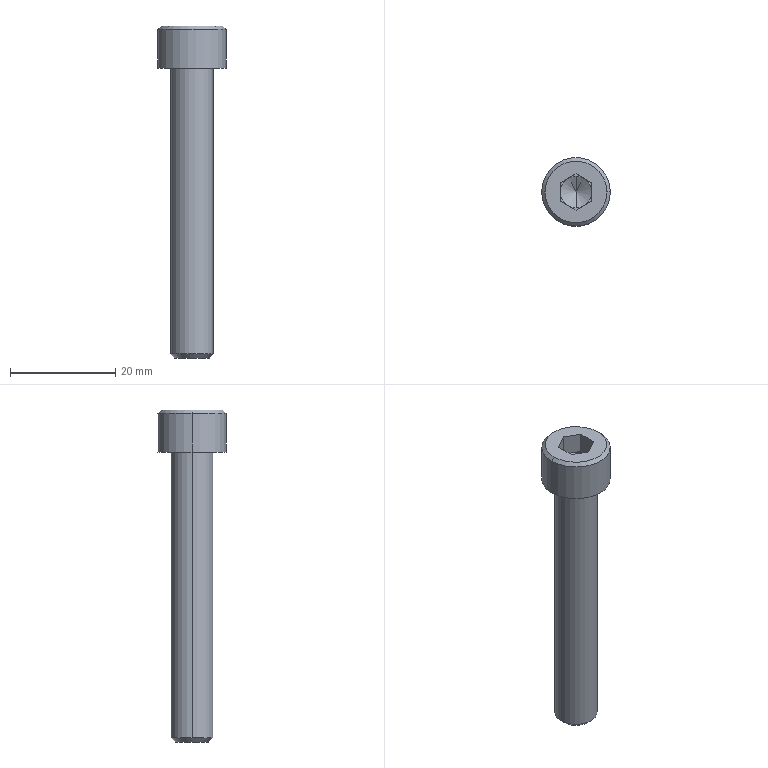Part | STEP file | 001-006-TAC01_M8_L55 | 1 solid | 25 faces | box 13 x 13 x 63 mm | volume 3670 mm3 | plane 15 | cone 6 | cylinder 4 | commonest cylinder face diameters 8 x2 13 x2